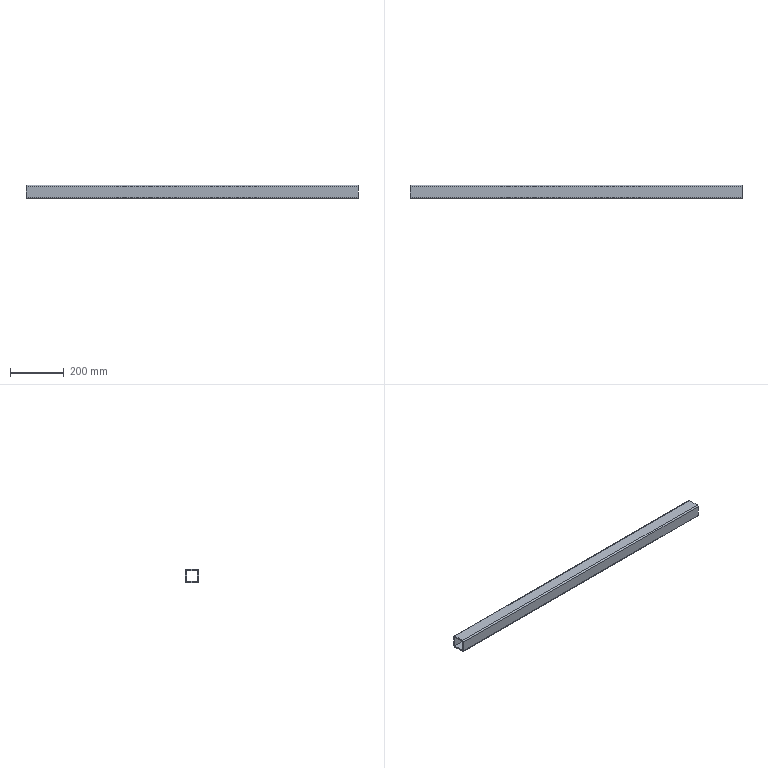Part | STEP file | 50x50x1240 | 1 solid | 14 faces | box 1240 x 50 x 50 mm | volume 1089389 mm3 | plane 10 | cylinder 4 | commonest cylinder face diameters 10 x4
STEP:
#1=CARTESIAN_POINT('',(0.,0.,0.));
#2=DIRECTION('',(0.,0.,1.));
#3=DIRECTION('',(1.,0.,0.));
#4=AXIS2_PLACEMENT_3D('',#1,#2,#3);
#5=CARTESIAN_POINT('',(-803.5,420.,-65.));
#6=VERTEX_POINT('',#5);
#7=CARTESIAN_POINT('',(-803.5,420.,-25.));
#8=VERTEX_POINT('',#7);
#9=CARTESIAN_POINT('',(-803.5,420.,-25.));
#10=DIRECTION('',(0.,0.,1.));
#11=VECTOR('',#10,1.);
#12=LINE('',#9,#11);
#13=CARTESIAN_POINT('',(636.5,420.,-25.));
#14=DIRECTION('',(0.,-1.,0.));
#15=DIRECTION('',(0.,0.,1.));
#16=AXIS2_PLACEMENT_3D('',#13,#14,#15);
#17=PLANE('',#16);
#18=CARTESIAN_POINT('',(0.,1440.));
#19=DIRECTION('',(1.,0.));
#20=VECTOR('',#19,1.);
#21=LINE('',#18,#20);
#22=(GEOMETRIC_REPRESENTATION_CONTEXT(2)PARAMETRIC_REPRESENTATION_CONTEXT()REPRESENTATION_CONTEXT('',''));
#23=DEFINITIONAL_REPRESENTATION('',(#21),#22);
#24=PCURVE('',#17,#23);
#25=CARTESIAN_POINT('',(-803.5,375.,-20.));
#26=DIRECTION('',(-1.,0.,0.));
#27=DIRECTION('',(0.,0.,1.));
#28=AXIS2_PLACEMENT_3D('',#25,#26,#27);
#29=PLANE('',#28);
#30=CARTESIAN_POINT('',(-5.,45.));
#31=DIRECTION('',(1.,0.));
#32=VECTOR('',#31,1.);
#33=LINE('',#30,#32);
#34=(GEOMETRIC_REPRESENTATION_CONTEXT(2)PARAMETRIC_REPRESENTATION_CONTEXT()REPRESENTATION_CONTEXT('',''));
#35=DEFINITIONAL_REPRESENTATION('',(#33),#34);
#36=PCURVE('',#29,#35);
#37=SURFACE_CURVE('',#12,(#24,#36),.PCURVE_S1.);
#38=EDGE_CURVE('',#6,#8,#37,.T.);
#39=ORIENTED_EDGE('',*,*,#38,.F.);
#40=CARTESIAN_POINT('',(436.5,420.,-65.));
#41=VERTEX_POINT('',#40);
#42=CARTESIAN_POINT('',(636.5,420.,-65.));
#43=DIRECTION('',(1.,0.,0.));
#44=VECTOR('',#43,1.);
#45=LINE('',#42,#44);
#46=CARTESIAN_POINT('',(-40.,0.));
#47=DIRECTION('',(0.,-1.));
#48=VECTOR('',#47,1.);
#49=LINE('',#46,#48);
#50=(GEOMETRIC_REPRESENTATION_CONTEXT(2)PARAMETRIC_REPRESENTATION_CONTEXT()REPRESENTATION_CONTEXT('',''));
#51=DEFINITIONAL_REPRESENTATION('',(#49),#50);
#52=PCURVE('',#17,#51);
#53=CARTESIAN_POINT('',(636.5,420.,-65.));
#54=DIRECTION('',(0.,0.,1.));
#55=DIRECTION('',(0.,1.,0.));
#56=AXIS2_PLACEMENT_3D('',#53,#54,#55);
#57=PLANE('',#56);
#58=CARTESIAN_POINT('',(0.,0.));
#59=DIRECTION('',(0.,-1.));
#60=VECTOR('',#59,1.);
#61=LINE('',#58,#60);
#62=(GEOMETRIC_REPRESENTATION_CONTEXT(2)PARAMETRIC_REPRESENTATION_CONTEXT()REPRESENTATION_CONTEXT('',''));
#63=DEFINITIONAL_REPRESENTATION('',(#61),#62);
#64=PCURVE('',#57,#63);
#65=SURFACE_CURVE('',#45,(#52,#64),.PCURVE_S1.);
#66=EDGE_CURVE('',#6,#41,#65,.T.);
#67=ORIENTED_EDGE('',*,*,#66,.T.);
#68=CARTESIAN_POINT('',(436.5,420.,-25.));
#69=VERTEX_POINT('',#68);
#70=CARTESIAN_POINT('',(436.5,420.,-25.));
#71=DIRECTION('',(0.,0.,1.));
#72=VECTOR('',#71,1.);
#73=LINE('',#70,#72);
#74=CARTESIAN_POINT('',(0.,200.));
#75=DIRECTION('',(1.,0.));
#76=VECTOR('',#75,1.);
#77=LINE('',#74,#76);
#78=(GEOMETRIC_REPRESENTATION_CONTEXT(2)PARAMETRIC_REPRESENTATION_CONTEXT()REPRESENTATION_CONTEXT('',''));
#79=DEFINITIONAL_REPRESENTATION('',(#77),#78);
#80=PCURVE('',#17,#79);
#81=CARTESIAN_POINT('',(436.5,420.,-670.));
#82=DIRECTION('',(-1.,0.,0.));
#83=DIRECTION('',(0.,0.,1.));
#84=AXIS2_PLACEMENT_3D('',#81,#82,#83);
#85=PLANE('',#84);
#86=CARTESIAN_POINT('',(645.,0.));
#87=DIRECTION('',(1.,0.));
#88=VECTOR('',#87,1.);
#89=LINE('',#86,#88);
#90=(GEOMETRIC_REPRESENTATION_CONTEXT(2)PARAMETRIC_REPRESENTATION_CONTEXT()REPRESENTATION_CONTEXT('',''));
#91=DEFINITIONAL_REPRESENTATION('',(#89),#90);
#92=PCURVE('',#85,#91);
#93=SURFACE_CURVE('',#73,(#80,#92),.PCURVE_S1.);
#94=EDGE_CURVE('',#41,#69,#93,.T.);
#95=ORIENTED_EDGE('',*,*,#94,.T.);
#96=CARTESIAN_POINT('',(636.5,420.,-25.));
#97=DIRECTION('',(1.,0.,0.));
#98=VECTOR('',#97,1.);
#99=LINE('',#96,#98);
#100=CARTESIAN_POINT('',(0.,0.));
#101=DIRECTION('',(0.,-1.));
#102=VECTOR('',#101,1.);
#103=LINE('',#100,#102);
#104=(GEOMETRIC_REPRESENTATION_CONTEXT(2)PARAMETRIC_REPRESENTATION_CONTEXT()REPRESENTATION_CONTEXT('',''));
#105=DEFINITIONAL_REPRESENTATION('',(#103),#104);
#106=PCURVE('',#17,#105);
#107=CARTESIAN_POINT('',(636.5,380.,-25.));
#108=DIRECTION('',(0.,0.,-1.));
#109=DIRECTION('',(0.,-1.,0.));
#110=AXIS2_PLACEMENT_3D('',#107,#108,#109);
#111=PLANE('',#110);
#112=CARTESIAN_POINT('',(-40.,0.));
#113=DIRECTION('',(0.,-1.));
#114=VECTOR('',#113,1.);
#115=LINE('',#112,#114);
#116=(GEOMETRIC_REPRESENTATION_CONTEXT(2)PARAMETRIC_REPRESENTATION_CONTEXT()REPRESENTATION_CONTEXT('',''));
#117=DEFINITIONAL_REPRESENTATION('',(#115),#116);
#118=PCURVE('',#111,#117);
#119=SURFACE_CURVE('',#99,(#106,#118),.PCURVE_S1.);
#120=EDGE_CURVE('',#8,#69,#119,.T.);
#121=ORIENTED_EDGE('',*,*,#120,.F.);
#122=EDGE_LOOP('',(#39,#67,#95,#121));
#123=FACE_BOUND('',#122,.T.);
#124=ADVANCED_FACE('',(#123),#17,.T.);
#125=CARTESIAN_POINT('',(-803.5,380.,-25.));
#126=VERTEX_POINT('',#125);
#127=CARTESIAN_POINT('',(-803.5,380.,-25.));
#128=DIRECTION('',(0.,-1.,0.));
#129=VECTOR('',#128,1.);
#130=LINE('',#127,#129);
#131=CARTESIAN_POINT('',(0.,1440.));
#132=DIRECTION('',(1.,0.));
#133=VECTOR('',#132,1.);
#134=LINE('',#131,#133);
#135=(GEOMETRIC_REPRESENTATION_CONTEXT(2)PARAMETRIC_REPRESENTATION_CONTEXT()REPRESENTATION_CONTEXT('',''));
#136=DEFINITIONAL_REPRESENTATION('',(#134),#135);
#137=PCURVE('',#111,#136);
#138=CARTESIAN_POINT('',(-5.,5.));
#139=DIRECTION('',(0.,-1.));
#140=VECTOR('',#139,1.);
#141=LINE('',#138,#140);
#142=(GEOMETRIC_REPRESENTATION_CONTEXT(2)PARAMETRIC_REPRESENTATION_CONTEXT()REPRESENTATION_CONTEXT('',''));
#143=DEFINITIONAL_REPRESENTATION('',(#141),#142);
#144=PCURVE('',#29,#143);
#145=SURFACE_CURVE('',#130,(#137,#144),.PCURVE_S1.);
#146=EDGE_CURVE('',#8,#126,#145,.T.);
#147=ORIENTED_EDGE('',*,*,#146,.F.);
#148=ORIENTED_EDGE('',*,*,#120,.T.);
#149=CARTESIAN_POINT('',(436.5,380.,-25.));
#150=VERTEX_POINT('',#149);
#151=CARTESIAN_POINT('',(436.5,380.,-25.));
#152=DIRECTION('',(0.,-1.,0.));
#153=VECTOR('',#152,1.);
#154=LINE('',#151,#153);
#155=CARTESIAN_POINT('',(0.,200.));
#156=DIRECTION('',(1.,0.));
#157=VECTOR('',#156,1.);
#158=LINE('',#155,#157);
#159=(GEOMETRIC_REPRESENTATION_CONTEXT(2)PARAMETRIC_REPRESENTATION_CONTEXT()REPRESENTATION_CONTEXT('',''));
#160=DEFINITIONAL_REPRESENTATION('',(#158),#159);
#161=PCURVE('',#111,#160);
#162=CARTESIAN_POINT('',(645.,-40.));
#163=DIRECTION('',(0.,-1.));
#164=VECTOR('',#163,1.);
#165=LINE('',#162,#164);
#166=(GEOMETRIC_REPRESENTATION_CONTEXT(2)PARAMETRIC_REPRESENTATION_CONTEXT()REPRESENTATION_CONTEXT('',''));
#167=DEFINITIONAL_REPRESENTATION('',(#165),#166);
#168=PCURVE('',#85,#167);
#169=SURFACE_CURVE('',#154,(#161,#168),.PCURVE_S1.);
#170=EDGE_CURVE('',#69,#150,#169,.T.);
#171=ORIENTED_EDGE('',*,*,#170,.T.);
#172=CARTESIAN_POINT('',(636.5,380.,-25.));
#173=DIRECTION('',(1.,0.,0.));
#174=VECTOR('',#173,1.);
#175=LINE('',#172,#174);
#176=CARTESIAN_POINT('',(0.,0.));
#177=DIRECTION('',(0.,-1.));
#178=VECTOR('',#177,1.);
#179=LINE('',#176,#178);
#180=(GEOMETRIC_REPRESENTATION_CONTEXT(2)PARAMETRIC_REPRESENTATION_CONTEXT()REPRESENTATION_CONTEXT('',''));
#181=DEFINITIONAL_REPRESENTATION('',(#179),#180);
#182=PCURVE('',#111,#181);
#183=CARTESIAN_POINT('',(636.5,380.,-65.));
#184=DIRECTION('',(0.,1.,0.));
#185=DIRECTION('',(0.,0.,-1.));
#186=AXIS2_PLACEMENT_3D('',#183,#184,#185);
#187=PLANE('',#186);
#188=CARTESIAN_POINT('',(-40.,0.));
#189=DIRECTION('',(0.,-1.));
#190=VECTOR('',#189,1.);
#191=LINE('',#188,#190);
#192=(GEOMETRIC_REPRESENTATION_CONTEXT(2)PARAMETRIC_REPRESENTATION_CONTEXT()REPRESENTATION_CONTEXT('',''));
#193=DEFINITIONAL_REPRESENTATION('',(#191),#192);
#194=PCURVE('',#187,#193);
#195=SURFACE_CURVE('',#175,(#182,#194),.PCURVE_S1.);
#196=EDGE_CURVE('',#126,#150,#195,.T.);
#197=ORIENTED_EDGE('',*,*,#196,.F.);
#198=EDGE_LOOP('',(#147,#148,#171,#197));
#199=FACE_BOUND('',#198,.T.);
#200=ADVANCED_FACE('',(#199),#111,.T.);
#201=CARTESIAN_POINT('',(-803.5,380.,-65.));
#202=VERTEX_POINT('',#201);
#203=CARTESIAN_POINT('',(-803.5,380.,-65.));
#204=DIRECTION('',(0.,0.,-1.));
#205=VECTOR('',#204,1.);
#206=LINE('',#203,#205);
#207=CARTESIAN_POINT('',(0.,1440.));
#208=DIRECTION('',(1.,0.));
#209=VECTOR('',#208,1.);
#210=LINE('',#207,#209);
#211=(GEOMETRIC_REPRESENTATION_CONTEXT(2)PARAMETRIC_REPRESENTATION_CONTEXT()REPRESENTATION_CONTEXT('',''));
#212=DEFINITIONAL_REPRESENTATION('',(#210),#211);
#213=PCURVE('',#187,#212);
#214=CARTESIAN_POINT('',(-45.,5.));
#215=DIRECTION('',(-1.,0.));
#216=VECTOR('',#215,1.);
#217=LINE('',#214,#216);
#218=(GEOMETRIC_REPRESENTATION_CONTEXT(2)PARAMETRIC_REPRESENTATION_CONTEXT()REPRESENTATION_CONTEXT('',''));
#219=DEFINITIONAL_REPRESENTATION('',(#217),#218);
#220=PCURVE('',#29,#219);
#221=SURFACE_CURVE('',#206,(#213,#220),.PCURVE_S1.);
#222=EDGE_CURVE('',#126,#202,#221,.T.);
#223=ORIENTED_EDGE('',*,*,#222,.F.);
#224=ORIENTED_EDGE('',*,*,#196,.T.);
#225=CARTESIAN_POINT('',(436.5,380.,-65.));
#226=VERTEX_POINT('',#225);
#227=CARTESIAN_POINT('',(436.5,380.,-65.));
#228=DIRECTION('',(0.,0.,-1.));
#229=VECTOR('',#228,1.);
#230=LINE('',#227,#229);
#231=CARTESIAN_POINT('',(0.,200.));
#232=DIRECTION('',(1.,0.));
#233=VECTOR('',#232,1.);
#234=LINE('',#231,#233);
#235=(GEOMETRIC_REPRESENTATION_CONTEXT(2)PARAMETRIC_REPRESENTATION_CONTEXT()REPRESENTATION_CONTEXT('',''));
#236=DEFINITIONAL_REPRESENTATION('',(#234),#235);
#237=PCURVE('',#187,#236);
#238=CARTESIAN_POINT('',(605.,-40.));
#239=DIRECTION('',(-1.,0.));
#240=VECTOR('',#239,1.);
#241=LINE('',#238,#240);
#242=(GEOMETRIC_REPRESENTATION_CONTEXT(2)PARAMETRIC_REPRESENTATION_CONTEXT()REPRESENTATION_CONTEXT('',''));
#243=DEFINITIONAL_REPRESENTATION('',(#241),#242);
#244=PCURVE('',#85,#243);
#245=SURFACE_CURVE('',#230,(#237,#244),.PCURVE_S1.);
#246=EDGE_CURVE('',#150,#226,#245,.T.);
#247=ORIENTED_EDGE('',*,*,#246,.T.);
#248=CARTESIAN_POINT('',(636.5,380.,-65.));
#249=DIRECTION('',(1.,0.,0.));
#250=VECTOR('',#249,1.);
#251=LINE('',#248,#250);
#252=CARTESIAN_POINT('',(0.,0.));
#253=DIRECTION('',(0.,-1.));
#254=VECTOR('',#253,1.);
#255=LINE('',#252,#254);
#256=(GEOMETRIC_REPRESENTATION_CONTEXT(2)PARAMETRIC_REPRESENTATION_CONTEXT()REPRESENTATION_CONTEXT('',''));
#257=DEFINITIONAL_REPRESENTATION('',(#255),#256);
#258=PCURVE('',#187,#257);
#259=CARTESIAN_POINT('',(-40.,0.));
#260=DIRECTION('',(0.,-1.));
#261=VECTOR('',#260,1.);
#262=LINE('',#259,#261);
#263=(GEOMETRIC_REPRESENTATION_CONTEXT(2)PARAMETRIC_REPRESENTATION_CONTEXT()REPRESENTATION_CONTEXT('',''));
#264=DEFINITIONAL_REPRESENTATION('',(#262),#263);
#265=PCURVE('',#57,#264);
#266=SURFACE_CURVE('',#251,(#258,#265),.PCURVE_S1.);
#267=EDGE_CURVE('',#202,#226,#266,.T.);
#268=ORIENTED_EDGE('',*,*,#267,.F.);
#269=EDGE_LOOP('',(#223,#224,#247,#268));
#270=FACE_BOUND('',#269,.T.);
#271=ADVANCED_FACE('',(#270),#187,.T.);
#272=CARTESIAN_POINT('',(-803.5,425.,-65.));
#273=VERTEX_POINT('',#272);
#274=CARTESIAN_POINT('',(-803.5,425.,-25.));
#275=VERTEX_POINT('',#274);
#276=CARTESIAN_POINT('',(-803.5,425.,-25.));
#277=DIRECTION('',(0.,0.,1.));
#278=VECTOR('',#277,1.);
#279=LINE('',#276,#278);
#280=CARTESIAN_POINT('',(636.5,425.,-25.));
#281=DIRECTION('',(0.,-1.,0.));
#282=DIRECTION('',(0.,0.,1.));
#283=AXIS2_PLACEMENT_3D('',#280,#281,#282);
#284=PLANE('',#283);
#285=CARTESIAN_POINT('',(0.,1440.));
#286=DIRECTION('',(1.,0.));
#287=VECTOR('',#286,1.);
#288=LINE('',#285,#287);
#289=(GEOMETRIC_REPRESENTATION_CONTEXT(2)PARAMETRIC_REPRESENTATION_CONTEXT()REPRESENTATION_CONTEXT('',''));
#290=DEFINITIONAL_REPRESENTATION('',(#288),#289);
#291=PCURVE('',#284,#290);
#292=CARTESIAN_POINT('',(-5.,50.));
#293=DIRECTION('',(1.,0.));
#294=VECTOR('',#293,1.);
#295=LINE('',#292,#294);
#296=(GEOMETRIC_REPRESENTATION_CONTEXT(2)PARAMETRIC_REPRESENTATION_CONTEXT()REPRESENTATION_CONTEXT('',''));
#297=DEFINITIONAL_REPRESENTATION('',(#295),#296);
#298=PCURVE('',#29,#297);
#299=SURFACE_CURVE('',#279,(#291,#298),.PCURVE_S1.);
#300=EDGE_CURVE('',#273,#275,#299,.T.);
#301=ORIENTED_EDGE('',*,*,#300,.T.);
#302=CARTESIAN_POINT('',(436.5,425.,-25.));
#303=VERTEX_POINT('',#302);
#304=CARTESIAN_POINT('',(636.5,425.,-25.));
#305=DIRECTION('',(1.,0.,0.));
#306=VECTOR('',#305,1.);
#307=LINE('',#304,#306);
#308=CARTESIAN_POINT('',(0.,0.));
#309=DIRECTION('',(0.,-1.));
#310=VECTOR('',#309,1.);
#311=LINE('',#308,#310);
#312=(GEOMETRIC_REPRESENTATION_CONTEXT(2)PARAMETRIC_REPRESENTATION_CONTEXT()REPRESENTATION_CONTEXT('',''));
#313=DEFINITIONAL_REPRESENTATION('',(#311),#312);
#314=PCURVE('',#284,#313);
#315=CARTESIAN_POINT('',(636.5,420.,-25.));
#316=DIRECTION('',(-1.,0.,0.));
#317=DIRECTION('',(0.,0.,1.));
#318=AXIS2_PLACEMENT_3D('',#315,#316,#317);
#319=CYLINDRICAL_SURFACE('',#318,5.);
#320=CARTESIAN_POINT('',(1.571,0.));
#321=DIRECTION('',(0.,-1.));
#322=VECTOR('',#321,1.);
#323=LINE('',#320,#322);
#324=(GEOMETRIC_REPRESENTATION_CONTEXT(2)PARAMETRIC_REPRESENTATION_CONTEXT()REPRESENTATION_CONTEXT('',''));
#325=DEFINITIONAL_REPRESENTATION('',(#323),#324);
#326=PCURVE('',#319,#325);
#327=SURFACE_CURVE('',#307,(#314,#326),.PCURVE_S1.);
#328=EDGE_CURVE('',#275,#303,#327,.T.);
#329=ORIENTED_EDGE('',*,*,#328,.T.);
#330=CARTESIAN_POINT('',(436.5,425.,-65.));
#331=VERTEX_POINT('',#330);
#332=CARTESIAN_POINT('',(436.5,425.,-25.));
#333=DIRECTION('',(0.,0.,1.));
#334=VECTOR('',#333,1.);
#335=LINE('',#332,#334);
#336=CARTESIAN_POINT('',(0.,200.));
#337=DIRECTION('',(1.,0.));
#338=VECTOR('',#337,1.);
#339=LINE('',#336,#338);
#340=(GEOMETRIC_REPRESENTATION_CONTEXT(2)PARAMETRIC_REPRESENTATION_CONTEXT()REPRESENTATION_CONTEXT('',''));
#341=DEFINITIONAL_REPRESENTATION('',(#339),#340);
#342=PCURVE('',#284,#341);
#343=CARTESIAN_POINT('',(645.,5.));
#344=DIRECTION('',(1.,0.));
#345=VECTOR('',#344,1.);
#346=LINE('',#343,#345);
#347=(GEOMETRIC_REPRESENTATION_CONTEXT(2)PARAMETRIC_REPRESENTATION_CONTEXT()REPRESENTATION_CONTEXT('',''));
#348=DEFINITIONAL_REPRESENTATION('',(#346),#347);
#349=PCURVE('',#85,#348);
#350=SURFACE_CURVE('',#335,(#342,#349),.PCURVE_S1.);
#351=EDGE_CURVE('',#331,#303,#350,.T.);
#352=ORIENTED_EDGE('',*,*,#351,.F.);
#353=CARTESIAN_POINT('',(636.5,425.,-65.));
#354=DIRECTION('',(1.,0.,0.));
#355=VECTOR('',#354,1.);
#356=LINE('',#353,#355);
#357=CARTESIAN_POINT('',(-40.,0.));
#358=DIRECTION('',(0.,-1.));
#359=VECTOR('',#358,1.);
#360=LINE('',#357,#359);
#361=(GEOMETRIC_REPRESENTATION_CONTEXT(2)PARAMETRIC_REPRESENTATION_CONTEXT()REPRESENTATION_CONTEXT('',''));
#362=DEFINITIONAL_REPRESENTATION('',(#360),#361);
#363=PCURVE('',#284,#362);
#364=CARTESIAN_POINT('',(636.5,420.,-65.));
#365=DIRECTION('',(-1.,0.,0.));
#366=DIRECTION('',(0.,0.,1.));
#367=AXIS2_PLACEMENT_3D('',#364,#365,#366);
#368=CYLINDRICAL_SURFACE('',#367,5.);
#369=CARTESIAN_POINT('',(1.571,0.));
#370=DIRECTION('',(0.,-1.));
#371=VECTOR('',#370,1.);
#372=LINE('',#369,#371);
#373=(GEOMETRIC_REPRESENTATION_CONTEXT(2)PARAMETRIC_REPRESENTATION_CONTEXT()REPRESENTATION_CONTEXT('',''));
#374=DEFINITIONAL_REPRESENTATION('',(#372),#373);
#375=PCURVE('',#368,#374);
#376=SURFACE_CURVE('',#356,(#363,#375),.PCURVE_S1.);
#377=EDGE_CURVE('',#273,#331,#376,.T.);
#378=ORIENTED_EDGE('',*,*,#377,.F.);
#379=EDGE_LOOP('',(#301,#329,#352,#378));
#380=FACE_BOUND('',#379,.T.);
#381=ADVANCED_FACE('',(#380),#284,.F.);
#382=CARTESIAN_POINT('',(-803.5,420.,-70.));
#383=VERTEX_POINT('',#382);
#384=CARTESIAN_POINT('',(-803.5,420.,-65.));
#385=DIRECTION('',(1.,0.,0.));
#386=DIRECTION('',(0.,0.,1.));
#387=AXIS2_PLACEMENT_3D('',#384,#385,#386);
#388=CIRCLE('',#387,5.);
#389=CARTESIAN_POINT('',(6.283,1440.));
#390=DIRECTION('',(-1.,0.));
#391=VECTOR('',#390,1.);
#392=LINE('',#389,#391);
#393=(GEOMETRIC_REPRESENTATION_CONTEXT(2)PARAMETRIC_REPRESENTATION_CONTEXT()REPRESENTATION_CONTEXT('',''));
#394=DEFINITIONAL_REPRESENTATION('',(#392),#393);
#395=PCURVE('',#368,#394);
#396=CARTESIAN_POINT('',(-40.,45.));
#397=CARTESIAN_POINT('',(-40.,36.34));
#398=CARTESIAN_POINT('',(-47.5,40.67));
#399=CARTESIAN_POINT('',(-55.,45.));
#400=CARTESIAN_POINT('',(-47.5,49.33));
#401=CARTESIAN_POINT('',(-40.,53.66));
#402=CARTESIAN_POINT('',(-40.,45.));
#403=(BOUNDED_CURVE()B_SPLINE_CURVE(2,(#396,#397,#398,#399,#400,#401,#402),.UNSPECIFIED.,.T.,.F.)B_SPLINE_CURVE_WITH_KNOTS((1,2,2,2,2,1),(-2.094,0.,2.094,4.189,6.283,8.378),.UNSPECIFIED.)CURVE()GEOMETRIC_REPRESENTATION_ITEM()RATIONAL_B_SPLINE_CURVE((1.,0.5,1.,0.5,1.,0.5,1.))REPRESENTATION_ITEM(''));
#404=(GEOMETRIC_REPRESENTATION_CONTEXT(2)PARAMETRIC_REPRESENTATION_CONTEXT()REPRESENTATION_CONTEXT('',''));
#405=DEFINITIONAL_REPRESENTATION('',(#403),#404);
#406=PCURVE('',#29,#405);
#407=SURFACE_CURVE('',#388,(#395,#406),.PCURVE_S1.);
#408=EDGE_CURVE('',#383,#273,#407,.T.);
#409=ORIENTED_EDGE('',*,*,#408,.T.);
#410=ORIENTED_EDGE('',*,*,#377,.T.);
#411=CARTESIAN_POINT('',(436.5,420.,-70.));
#412=VERTEX_POINT('',#411);
#413=CARTESIAN_POINT('',(436.5,420.,-65.));
#414=DIRECTION('',(1.,0.,0.));
#415=DIRECTION('',(0.,0.,1.));
#416=AXIS2_PLACEMENT_3D('',#413,#414,#415);
#417=CIRCLE('',#416,5.);
#418=CARTESIAN_POINT('',(6.283,200.));
#419=DIRECTION('',(-1.,0.));
#420=VECTOR('',#419,1.);
#421=LINE('',#418,#420);
#422=(GEOMETRIC_REPRESENTATION_CONTEXT(2)PARAMETRIC_REPRESENTATION_CONTEXT()REPRESENTATION_CONTEXT('',''));
#423=DEFINITIONAL_REPRESENTATION('',(#421),#422);
#424=PCURVE('',#368,#423);
#425=CARTESIAN_POINT('',(610.,0.));
#426=CARTESIAN_POINT('',(610.,-8.66));
#427=CARTESIAN_POINT('',(602.5,-4.33));
#428=CARTESIAN_POINT('',(595.,0.));
#429=CARTESIAN_POINT('',(602.5,4.33));
#430=CARTESIAN_POINT('',(610.,8.66));
#431=CARTESIAN_POINT('',(610.,0.));
#432=(BOUNDED_CURVE()B_SPLINE_CURVE(2,(#425,#426,#427,#428,#429,#430,#431),.UNSPECIFIED.,.T.,.F.)B_SPLINE_CURVE_WITH_KNOTS((1,2,2,2,2,1),(-2.094,0.,2.094,4.189,6.283,8.378),.UNSPECIFIED.)CURVE()GEOMETRIC_REPRESENTATION_ITEM()RATIONAL_B_SPLINE_CURVE((1.,0.5,1.,0.5,1.,0.5,1.))REPRESENTATION_ITEM(''));
#433=(GEOMETRIC_REPRESENTATION_CONTEXT(2)PARAMETRIC_REPRESENTATION_CONTEXT()REPRESENTATION_CONTEXT('',''));
#434=DEFINITIONAL_REPRESENTATION('',(#432),#433);
#435=PCURVE('',#85,#434);
#436=SURFACE_CURVE('',#417,(#424,#435),.PCURVE_S1.);
#437=EDGE_CURVE('',#412,#331,#436,.T.);
#438=ORIENTED_EDGE('',*,*,#437,.F.);
#439=CARTESIAN_POINT('',(636.5,420.,-70.));
#440=DIRECTION('',(1.,0.,0.));
#441=VECTOR('',#440,1.);
#442=LINE('',#439,#441);
#443=CARTESIAN_POINT('',(3.142,0.));
#444=DIRECTION('',(0.,-1.));
#445=VECTOR('',#444,1.);
#446=LINE('',#443,#445);
#447=(GEOMETRIC_REPRESENTATION_CONTEXT(2)PARAMETRIC_REPRESENTATION_CONTEXT()REPRESENTATION_CONTEXT('',''));
#448=DEFINITIONAL_REPRESENTATION('',(#446),#447);
#449=PCURVE('',#368,#448);
#450=CARTESIAN_POINT('',(636.5,420.,-70.));
#451=DIRECTION('',(0.,0.,1.));
#452=DIRECTION('',(0.,1.,0.));
#453=AXIS2_PLACEMENT_3D('',#450,#451,#452);
#454=PLANE('',#453);
#455=CARTESIAN_POINT('',(0.,0.));
#456=DIRECTION('',(0.,-1.));
#457=VECTOR('',#456,1.);
#458=LINE('',#455,#457);
#459=(GEOMETRIC_REPRESENTATION_CONTEXT(2)PARAMETRIC_REPRESENTATION_CONTEXT()REPRESENTATION_CONTEXT('',''));
#460=DEFINITIONAL_REPRESENTATION('',(#458),#459);
#461=PCURVE('',#454,#460);
#462=SURFACE_CURVE('',#442,(#449,#461),.PCURVE_S1.);
#463=EDGE_CURVE('',#383,#412,#462,.T.);
#464=ORIENTED_EDGE('',*,*,#463,.F.);
#465=EDGE_LOOP('',(#409,#410,#438,#464));
#466=FACE_BOUND('',#465,.T.);
#467=ADVANCED_FACE('',(#466),#368,.T.);
#468=CARTESIAN_POINT('',(-803.5,380.,-70.));
#469=VERTEX_POINT('',#468);
#470=CARTESIAN_POINT('',(-803.5,420.,-70.));
#471=DIRECTION('',(0.,1.,0.));
#472=VECTOR('',#471,1.);
#473=LINE('',#470,#472);
#474=CARTESIAN_POINT('',(0.,1440.));
#475=DIRECTION('',(1.,0.));
#476=VECTOR('',#475,1.);
#477=LINE('',#474,#476);
#478=(GEOMETRIC_REPRESENTATION_CONTEXT(2)PARAMETRIC_REPRESENTATION_CONTEXT()REPRESENTATION_CONTEXT('',''));
#479=DEFINITIONAL_REPRESENTATION('',(#477),#478);
#480=PCURVE('',#454,#479);
#481=CARTESIAN_POINT('',(-50.,45.));
#482=DIRECTION('',(0.,1.));
#483=VECTOR('',#482,1.);
#484=LINE('',#481,#483);
#485=(GEOMETRIC_REPRESENTATION_CONTEXT(2)PARAMETRIC_REPRESENTATION_CONTEXT()REPRESENTATION_CONTEXT('',''));
#486=DEFINITIONAL_REPRESENTATION('',(#484),#485);
#487=PCURVE('',#29,#486);
#488=SURFACE_CURVE('',#473,(#480,#487),.PCURVE_S1.);
#489=EDGE_CURVE('',#469,#383,#488,.T.);
#490=ORIENTED_EDGE('',*,*,#489,.T.);
#491=ORIENTED_EDGE('',*,*,#463,.T.);
#492=CARTESIAN_POINT('',(436.5,380.,-70.));
#493=VERTEX_POINT('',#492);
#494=CARTESIAN_POINT('',(436.5,420.,-70.));
#495=DIRECTION('',(0.,1.,0.));
#496=VECTOR('',#495,1.);
#497=LINE('',#494,#496);
#498=CARTESIAN_POINT('',(0.,200.));
#499=DIRECTION('',(1.,0.));
#500=VECTOR('',#499,1.);
#501=LINE('',#498,#500);
#502=(GEOMETRIC_REPRESENTATION_CONTEXT(2)PARAMETRIC_REPRESENTATION_CONTEXT()REPRESENTATION_CONTEXT('',''));
#503=DEFINITIONAL_REPRESENTATION('',(#501),#502);
#504=PCURVE('',#454,#503);
#505=CARTESIAN_POINT('',(600.,0.));
#506=DIRECTION('',(0.,1.));
#507=VECTOR('',#506,1.);
#508=LINE('',#505,#507);
#509=(GEOMETRIC_REPRESENTATION_CONTEXT(2)PARAMETRIC_REPRESENTATION_CONTEXT()REPRESENTATION_CONTEXT('',''));
#510=DEFINITIONAL_REPRESENTATION('',(#508),#509);
#511=PCURVE('',#85,#510);
#512=SURFACE_CURVE('',#497,(#504,#511),.PCURVE_S1.);
#513=EDGE_CURVE('',#493,#412,#512,.T.);
#514=ORIENTED_EDGE('',*,*,#513,.F.);
#515=CARTESIAN_POINT('',(636.5,380.,-70.));
#516=DIRECTION('',(1.,0.,0.));
#517=VECTOR('',#516,1.);
#518=LINE('',#515,#517);
#519=CARTESIAN_POINT('',(-40.,0.));
#520=DIRECTION('',(0.,-1.));
#521=VECTOR('',#520,1.);
#522=LINE('',#519,#521);
#523=(GEOMETRIC_REPRESENTATION_CONTEXT(2)PARAMETRIC_REPRESENTATION_CONTEXT()REPRESENTATION_CONTEXT('',''));
#524=DEFINITIONAL_REPRESENTATION('',(#522),#523);
#525=PCURVE('',#454,#524);
#526=CARTESIAN_POINT('',(636.5,380.,-65.));
#527=DIRECTION('',(-1.,0.,0.));
#528=DIRECTION('',(0.,0.,1.));
#529=AXIS2_PLACEMENT_3D('',#526,#527,#528);
#530=CYLINDRICAL_SURFACE('',#529,5.);
#531=CARTESIAN_POINT('',(3.142,0.));
#532=DIRECTION('',(0.,-1.));
#533=VECTOR('',#532,1.);
#534=LINE('',#531,#533);
#535=(GEOMETRIC_REPRESENTATION_CONTEXT(2)PARAMETRIC_REPRESENTATION_CONTEXT()REPRESENTATION_CONTEXT('',''));
#536=DEFINITIONAL_REPRESENTATION('',(#534),#535);
#537=PCURVE('',#530,#536);
#538=SURFACE_CURVE('',#518,(#525,#537),.PCURVE_S1.);
#539=EDGE_CURVE('',#469,#493,#538,.T.);
#540=ORIENTED_EDGE('',*,*,#539,.F.);
#541=EDGE_LOOP('',(#490,#491,#514,#540));
#542=FACE_BOUND('',#541,.T.);
#543=ADVANCED_FACE('',(#542),#454,.F.);
#544=CARTESIAN_POINT('',(-803.5,375.,-65.));
#545=VERTEX_POINT('',#544);
#546=CARTESIAN_POINT('',(-803.5,380.,-65.));
#547=DIRECTION('',(1.,0.,0.));
#548=DIRECTION('',(0.,0.,1.));
#549=AXIS2_PLACEMENT_3D('',#546,#547,#548);
#550=CIRCLE('',#549,5.);
#551=CARTESIAN_POINT('',(6.283,1440.));
#552=DIRECTION('',(-1.,0.));
#553=VECTOR('',#552,1.);
#554=LINE('',#551,#553);
#555=(GEOMETRIC_REPRESENTATION_CONTEXT(2)PARAMETRIC_REPRESENTATION_CONTEXT()REPRESENTATION_CONTEXT('',''));
#556=DEFINITIONAL_REPRESENTATION('',(#554),#555);
#557=PCURVE('',#530,#556);
#558=CARTESIAN_POINT('',(-40.,5.));
#559=CARTESIAN_POINT('',(-40.,-3.66));
#560=CARTESIAN_POINT('',(-47.5,0.6699));
#561=CARTESIAN_POINT('',(-55.,5.));
#562=CARTESIAN_POINT('',(-47.5,9.33));
#563=CARTESIAN_POINT('',(-40.,13.66));
#564=CARTESIAN_POINT('',(-40.,5.));
#565=(BOUNDED_CURVE()B_SPLINE_CURVE(2,(#558,#559,#560,#561,#562,#563,#564),.UNSPECIFIED.,.T.,.F.)B_SPLINE_CURVE_WITH_KNOTS((1,2,2,2,2,1),(-2.094,0.,2.094,4.189,6.283,8.378),.UNSPECIFIED.)CURVE()GEOMETRIC_REPRESENTATION_ITEM()RATIONAL_B_SPLINE_CURVE((1.,0.5,1.,0.5,1.,0.5,1.))REPRESENTATION_ITEM(''));
#566=(GEOMETRIC_REPRESENTATION_CONTEXT(2)PARAMETRIC_REPRESENTATION_CONTEXT()REPRESENTATION_CONTEXT('',''));
#567=DEFINITIONAL_REPRESENTATION('',(#565),#566);
#568=PCURVE('',#29,#567);
#569=SURFACE_CURVE('',#550,(#557,#568),.PCURVE_S1.);
#570=EDGE_CURVE('',#545,#469,#569,.T.);
#571=ORIENTED_EDGE('',*,*,#570,.T.);
#572=ORIENTED_EDGE('',*,*,#539,.T.);
#573=CARTESIAN_POINT('',(436.5,375.,-65.));
#574=VERTEX_POINT('',#573);
#575=CARTESIAN_POINT('',(436.5,380.,-65.));
#576=DIRECTION('',(1.,0.,0.));
#577=DIRECTION('',(0.,0.,1.));
#578=AXIS2_PLACEMENT_3D('',#575,#576,#577);
#579=CIRCLE('',#578,5.);
#580=CARTESIAN_POINT('',(6.283,200.));
#581=DIRECTION('',(-1.,0.));
#582=VECTOR('',#581,1.);
#583=LINE('',#580,#582);
#584=(GEOMETRIC_REPRESENTATION_CONTEXT(2)PARAMETRIC_REPRESENTATION_CONTEXT()REPRESENTATION_CONTEXT('',''));
#585=DEFINITIONAL_REPRESENTATION('',(#583),#584);
#586=PCURVE('',#530,#585);
#587=CARTESIAN_POINT('',(610.,-40.));
#588=CARTESIAN_POINT('',(610.,-48.66));
#589=CARTESIAN_POINT('',(602.5,-44.33));
#590=CARTESIAN_POINT('',(595.,-40.));
#591=CARTESIAN_POINT('',(602.5,-35.67));
#592=CARTESIAN_POINT('',(610.,-31.34));
#593=CARTESIAN_POINT('',(610.,-40.));
#594=(BOUNDED_CURVE()B_SPLINE_CURVE(2,(#587,#588,#589,#590,#591,#592,#593),.UNSPECIFIED.,.T.,.F.)B_SPLINE_CURVE_WITH_KNOTS((1,2,2,2,2,1),(-2.094,0.,2.094,4.189,6.283,8.378),.UNSPECIFIED.)CURVE()GEOMETRIC_REPRESENTATION_ITEM()RATIONAL_B_SPLINE_CURVE((1.,0.5,1.,0.5,1.,0.5,1.))REPRESENTATION_ITEM(''));
#595=(GEOMETRIC_REPRESENTATION_CONTEXT(2)PARAMETRIC_REPRESENTATION_CONTEXT()REPRESENTATION_CONTEXT('',''));
#596=DEFINITIONAL_REPRESENTATION('',(#594),#595);
#597=PCURVE('',#85,#596);
#598=SURFACE_CURVE('',#579,(#586,#597),.PCURVE_S1.);
#599=EDGE_CURVE('',#574,#493,#598,.T.);
#600=ORIENTED_EDGE('',*,*,#599,.F.);
#601=CARTESIAN_POINT('',(636.5,375.,-65.));
#602=DIRECTION('',(1.,0.,0.));
#603=VECTOR('',#602,1.);
#604=LINE('',#601,#603);
#605=CARTESIAN_POINT('',(4.712,0.));
#606=DIRECTION('',(0.,-1.));
#607=VECTOR('',#606,1.);
#608=LINE('',#605,#607);
#609=(GEOMETRIC_REPRESENTATION_CONTEXT(2)PARAMETRIC_REPRESENTATION_CONTEXT()REPRESENTATION_CONTEXT('',''));
#610=DEFINITIONAL_REPRESENTATION('',(#608),#609);
#611=PCURVE('',#530,#610);
#612=CARTESIAN_POINT('',(636.5,375.,-65.));
#613=DIRECTION('',(0.,1.,0.));
#614=DIRECTION('',(0.,0.,-1.));
#615=AXIS2_PLACEMENT_3D('',#612,#613,#614);
#616=PLANE('',#615);
#617=CARTESIAN_POINT('',(0.,0.));
#618=DIRECTION('',(0.,-1.));
#619=VECTOR('',#618,1.);
#620=LINE('',#617,#619);
#621=(GEOMETRIC_REPRESENTATION_CONTEXT(2)PARAMETRIC_REPRESENTATION_CONTEXT()REPRESENTATION_CONTEXT('',''));
#622=DEFINITIONAL_REPRESENTATION('',(#620),#621);
#623=PCURVE('',#616,#622);
#624=SURFACE_CURVE('',#604,(#611,#623),.PCURVE_S1.);
#625=EDGE_CURVE('',#545,#574,#624,.T.);
#626=ORIENTED_EDGE('',*,*,#625,.F.);
#627=EDGE_LOOP('',(#571,#572,#600,#626));
#628=FACE_BOUND('',#627,.T.);
#629=ADVANCED_FACE('',(#628),#530,.T.);
#630=CARTESIAN_POINT('',(-803.5,375.,-25.));
#631=VERTEX_POINT('',#630);
#632=CARTESIAN_POINT('',(-803.5,375.,-65.));
#633=DIRECTION('',(0.,0.,-1.));
#634=VECTOR('',#633,1.);
#635=LINE('',#632,#634);
#636=CARTESIAN_POINT('',(0.,1440.));
#637=DIRECTION('',(1.,0.));
#638=VECTOR('',#637,1.);
#639=LINE('',#636,#638);
#640=(GEOMETRIC_REPRESENTATION_CONTEXT(2)PARAMETRIC_REPRESENTATION_CONTEXT()REPRESENTATION_CONTEXT('',''));
#641=DEFINITIONAL_REPRESENTATION('',(#639),#640);
#642=PCURVE('',#616,#641);
#643=CARTESIAN_POINT('',(-45.,0.));
#644=DIRECTION('',(-1.,0.));
#645=VECTOR('',#644,1.);
#646=LINE('',#643,#645);
#647=(GEOMETRIC_REPRESENTATION_CONTEXT(2)PARAMETRIC_REPRESENTATION_CONTEXT()REPRESENTATION_CONTEXT('',''));
#648=DEFINITIONAL_REPRESENTATION('',(#646),#647);
#649=PCURVE('',#29,#648);
#650=SURFACE_CURVE('',#635,(#642,#649),.PCURVE_S1.);
#651=EDGE_CURVE('',#631,#545,#650,.T.);
#652=ORIENTED_EDGE('',*,*,#651,.T.);
#653=ORIENTED_EDGE('',*,*,#625,.T.);
#654=CARTESIAN_POINT('',(436.5,375.,-25.));
#655=VERTEX_POINT('',#654);
#656=CARTESIAN_POINT('',(436.5,375.,-65.));
#657=DIRECTION('',(0.,0.,-1.));
#658=VECTOR('',#657,1.);
#659=LINE('',#656,#658);
#660=CARTESIAN_POINT('',(0.,200.));
#661=DIRECTION('',(1.,0.));
#662=VECTOR('',#661,1.);
#663=LINE('',#660,#662);
#664=(GEOMETRIC_REPRESENTATION_CONTEXT(2)PARAMETRIC_REPRESENTATION_CONTEXT()REPRESENTATION_CONTEXT('',''));
#665=DEFINITIONAL_REPRESENTATION('',(#663),#664);
#666=PCURVE('',#616,#665);
#667=CARTESIAN_POINT('',(605.,-45.));
#668=DIRECTION('',(-1.,0.));
#669=VECTOR('',#668,1.);
#670=LINE('',#667,#669);
#671=(GEOMETRIC_REPRESENTATION_CONTEXT(2)PARAMETRIC_REPRESENTATION_CONTEXT()REPRESENTATION_CONTEXT('',''));
#672=DEFINITIONAL_REPRESENTATION('',(#670),#671);
#673=PCURVE('',#85,#672);
#674=SURFACE_CURVE('',#659,(#666,#673),.PCURVE_S1.);
#675=EDGE_CURVE('',#655,#574,#674,.T.);
#676=ORIENTED_EDGE('',*,*,#675,.F.);
#677=CARTESIAN_POINT('',(636.5,375.,-25.));
#678=DIRECTION('',(1.,0.,0.));
#679=VECTOR('',#678,1.);
#680=LINE('',#677,#679);
#681=CARTESIAN_POINT('',(-40.,0.));
#682=DIRECTION('',(0.,-1.));
#683=VECTOR('',#682,1.);
#684=LINE('',#681,#683);
#685=(GEOMETRIC_REPRESENTATION_CONTEXT(2)PARAMETRIC_REPRESENTATION_CONTEXT()REPRESENTATION_CONTEXT('',''));
#686=DEFINITIONAL_REPRESENTATION('',(#684),#685);
#687=PCURVE('',#616,#686);
#688=CARTESIAN_POINT('',(636.5,380.,-25.));
#689=DIRECTION('',(-1.,0.,0.));
#690=DIRECTION('',(0.,0.,1.));
#691=AXIS2_PLACEMENT_3D('',#688,#689,#690);
#692=CYLINDRICAL_SURFACE('',#691,5.);
#693=CARTESIAN_POINT('',(4.712,0.));
#694=DIRECTION('',(0.,-1.));
#695=VECTOR('',#694,1.);
#696=LINE('',#693,#695);
#697=(GEOMETRIC_REPRESENTATION_CONTEXT(2)PARAMETRIC_REPRESENTATION_CONTEXT()REPRESENTATION_CONTEXT('',''));
#698=DEFINITIONAL_REPRESENTATION('',(#696),#697);
#699=PCURVE('',#692,#698);
#700=SURFACE_CURVE('',#680,(#687,#699),.PCURVE_S1.);
#701=EDGE_CURVE('',#631,#655,#700,.T.);
#702=ORIENTED_EDGE('',*,*,#701,.F.);
#703=EDGE_LOOP('',(#652,#653,#676,#702));
#704=FACE_BOUND('',#703,.T.);
#705=ADVANCED_FACE('',(#704),#616,.F.);
#706=CARTESIAN_POINT('',(-803.5,380.,-20.));
#707=VERTEX_POINT('',#706);
#708=CARTESIAN_POINT('',(-803.5,380.,-25.));
#709=DIRECTION('',(1.,0.,0.));
#710=DIRECTION('',(0.,0.,1.));
#711=AXIS2_PLACEMENT_3D('',#708,#709,#710);
#712=CIRCLE('',#711,5.);
#713=CARTESIAN_POINT('',(6.283,1440.));
#714=DIRECTION('',(-1.,0.));
#715=VECTOR('',#714,1.);
#716=LINE('',#713,#715);
#717=(GEOMETRIC_REPRESENTATION_CONTEXT(2)PARAMETRIC_REPRESENTATION_CONTEXT()REPRESENTATION_CONTEXT('',''));
#718=DEFINITIONAL_REPRESENTATION('',(#716),#717);
#719=PCURVE('',#692,#718);
#720=CARTESIAN_POINT('',(0.,5.));
#721=CARTESIAN_POINT('',(0.,-3.66));
#722=CARTESIAN_POINT('',(-7.5,0.6699));
#723=CARTESIAN_POINT('',(-15.,5.));
#724=CARTESIAN_POINT('',(-7.5,9.33));
#725=CARTESIAN_POINT('',(0.,13.66));
#726=CARTESIAN_POINT('',(0.,5.));
#727=(BOUNDED_CURVE()B_SPLINE_CURVE(2,(#720,#721,#722,#723,#724,#725,#726),.UNSPECIFIED.,.T.,.F.)B_SPLINE_CURVE_WITH_KNOTS((1,2,2,2,2,1),(-2.094,0.,2.094,4.189,6.283,8.378),.UNSPECIFIED.)CURVE()GEOMETRIC_REPRESENTATION_ITEM()RATIONAL_B_SPLINE_CURVE((1.,0.5,1.,0.5,1.,0.5,1.))REPRESENTATION_ITEM(''));
#728=(GEOMETRIC_REPRESENTATION_CONTEXT(2)PARAMETRIC_REPRESENTATION_CONTEXT()REPRESENTATION_CONTEXT('',''));
#729=DEFINITIONAL_REPRESENTATION('',(#727),#728);
#730=PCURVE('',#29,#729);
#731=SURFACE_CURVE('',#712,(#719,#730),.PCURVE_S1.);
#732=EDGE_CURVE('',#707,#631,#731,.T.);
#733=ORIENTED_EDGE('',*,*,#732,.T.);
#734=ORIENTED_EDGE('',*,*,#701,.T.);
#735=CARTESIAN_POINT('',(436.5,380.,-20.));
#736=VERTEX_POINT('',#735);
#737=CARTESIAN_POINT('',(436.5,380.,-25.));
#738=DIRECTION('',(1.,0.,0.));
#739=DIRECTION('',(0.,0.,1.));
#740=AXIS2_PLACEMENT_3D('',#737,#738,#739);
#741=CIRCLE('',#740,5.);
#742=CARTESIAN_POINT('',(6.283,200.));
#743=DIRECTION('',(-1.,0.));
#744=VECTOR('',#743,1.);
#745=LINE('',#742,#744);
#746=(GEOMETRIC_REPRESENTATION_CONTEXT(2)PARAMETRIC_REPRESENTATION_CONTEXT()REPRESENTATION_CONTEXT('',''));
#747=DEFINITIONAL_REPRESENTATION('',(#745),#746);
#748=PCURVE('',#692,#747);
#749=CARTESIAN_POINT('',(650.,-40.));
#750=CARTESIAN_POINT('',(650.,-48.66));
#751=CARTESIAN_POINT('',(642.5,-44.33));
#752=CARTESIAN_POINT('',(635.,-40.));
#753=CARTESIAN_POINT('',(642.5,-35.67));
#754=CARTESIAN_POINT('',(650.,-31.34));
#755=CARTESIAN_POINT('',(650.,-40.));
#756=(BOUNDED_CURVE()B_SPLINE_CURVE(2,(#749,#750,#751,#752,#753,#754,#755),.UNSPECIFIED.,.T.,.F.)B_SPLINE_CURVE_WITH_KNOTS((1,2,2,2,2,1),(-2.094,0.,2.094,4.189,6.283,8.378),.UNSPECIFIED.)CURVE()GEOMETRIC_REPRESENTATION_ITEM()RATIONAL_B_SPLINE_CURVE((1.,0.5,1.,0.5,1.,0.5,1.))REPRESENTATION_ITEM(''));
#757=(GEOMETRIC_REPRESENTATION_CONTEXT(2)PARAMETRIC_REPRESENTATION_CONTEXT()REPRESENTATION_CONTEXT('',''));
#758=DEFINITIONAL_REPRESENTATION('',(#756),#757);
#759=PCURVE('',#85,#758);
#760=SURFACE_CURVE('',#741,(#748,#759),.PCURVE_S1.);
#761=EDGE_CURVE('',#736,#655,#760,.T.);
#762=ORIENTED_EDGE('',*,*,#761,.F.);
#763=CARTESIAN_POINT('',(636.5,380.,-20.));
#764=DIRECTION('',(1.,0.,0.));
#765=VECTOR('',#764,1.);
#766=LINE('',#763,#765);
#767=CARTESIAN_POINT('',(6.283,0.));
#768=DIRECTION('',(0.,-1.));
#769=VECTOR('',#768,1.);
#770=LINE('',#767,#769);
#771=(GEOMETRIC_REPRESENTATION_CONTEXT(2)PARAMETRIC_REPRESENTATION_CONTEXT()REPRESENTATION_CONTEXT('',''));
#772=DEFINITIONAL_REPRESENTATION('',(#770),#771);
#773=PCURVE('',#692,#772);
#774=CARTESIAN_POINT('',(636.5,380.,-20.));
#775=DIRECTION('',(0.,0.,-1.));
#776=DIRECTION('',(0.,-1.,0.));
#777=AXIS2_PLACEMENT_3D('',#774,#775,#776);
#778=PLANE('',#777);
#779=CARTESIAN_POINT('',(0.,0.));
#780=DIRECTION('',(0.,-1.));
#781=VECTOR('',#780,1.);
#782=LINE('',#779,#781);
#783=(GEOMETRIC_REPRESENTATION_CONTEXT(2)PARAMETRIC_REPRESENTATION_CONTEXT()REPRESENTATION_CONTEXT('',''));
#784=DEFINITIONAL_REPRESENTATION('',(#782),#783);
#785=PCURVE('',#778,#784);
#786=SURFACE_CURVE('',#766,(#773,#785),.PCURVE_S1.);
#787=EDGE_CURVE('',#707,#736,#786,.T.);
#788=ORIENTED_EDGE('',*,*,#787,.F.);
#789=EDGE_LOOP('',(#733,#734,#762,#788));
#790=FACE_BOUND('',#789,.T.);
#791=ADVANCED_FACE('',(#790),#692,.T.);
#792=CARTESIAN_POINT('',(-803.5,420.,-20.));
#793=VERTEX_POINT('',#792);
#794=CARTESIAN_POINT('',(-803.5,380.,-20.));
#795=DIRECTION('',(0.,-1.,0.));
#796=VECTOR('',#795,1.);
#797=LINE('',#794,#796);
#798=CARTESIAN_POINT('',(0.,1440.));
#799=DIRECTION('',(1.,0.));
#800=VECTOR('',#799,1.);
#801=LINE('',#798,#800);
#802=(GEOMETRIC_REPRESENTATION_CONTEXT(2)PARAMETRIC_REPRESENTATION_CONTEXT()REPRESENTATION_CONTEXT('',''));
#803=DEFINITIONAL_REPRESENTATION('',(#801),#802);
#804=PCURVE('',#778,#803);
#805=CARTESIAN_POINT('',(0.,5.));
#806=DIRECTION('',(0.,-1.));
#807=VECTOR('',#806,1.);
#808=LINE('',#805,#807);
#809=(GEOMETRIC_REPRESENTATION_CONTEXT(2)PARAMETRIC_REPRESENTATION_CONTEXT()REPRESENTATION_CONTEXT('',''));
#810=DEFINITIONAL_REPRESENTATION('',(#808),#809);
#811=PCURVE('',#29,#810);
#812=SURFACE_CURVE('',#797,(#804,#811),.PCURVE_S1.);
#813=EDGE_CURVE('',#793,#707,#812,.T.);
#814=ORIENTED_EDGE('',*,*,#813,.T.);
#815=ORIENTED_EDGE('',*,*,#787,.T.);
#816=CARTESIAN_POINT('',(436.5,420.,-20.));
#817=VERTEX_POINT('',#816);
#818=CARTESIAN_POINT('',(436.5,380.,-20.));
#819=DIRECTION('',(0.,-1.,0.));
#820=VECTOR('',#819,1.);
#821=LINE('',#818,#820);
#822=CARTESIAN_POINT('',(0.,200.));
#823=DIRECTION('',(1.,0.));
#824=VECTOR('',#823,1.);
#825=LINE('',#822,#824);
#826=(GEOMETRIC_REPRESENTATION_CONTEXT(2)PARAMETRIC_REPRESENTATION_CONTEXT()REPRESENTATION_CONTEXT('',''));
#827=DEFINITIONAL_REPRESENTATION('',(#825),#826);
#828=PCURVE('',#778,#827);
#829=CARTESIAN_POINT('',(650.,-40.));
#830=DIRECTION('',(0.,-1.));
#831=VECTOR('',#830,1.);
#832=LINE('',#829,#831);
#833=(GEOMETRIC_REPRESENTATION_CONTEXT(2)PARAMETRIC_REPRESENTATION_CONTEXT()REPRESENTATION_CONTEXT('',''));
#834=DEFINITIONAL_REPRESENTATION('',(#832),#833);
#835=PCURVE('',#85,#834);
#836=SURFACE_CURVE('',#821,(#828,#835),.PCURVE_S1.);
#837=EDGE_CURVE('',#817,#736,#836,.T.);
#838=ORIENTED_EDGE('',*,*,#837,.F.);
#839=CARTESIAN_POINT('',(636.5,420.,-20.));
#840=DIRECTION('',(1.,0.,0.));
#841=VECTOR('',#840,1.);
#842=LINE('',#839,#841);
#843=CARTESIAN_POINT('',(-40.,0.));
#844=DIRECTION('',(0.,-1.));
#845=VECTOR('',#844,1.);
#846=LINE('',#843,#845);
#847=(GEOMETRIC_REPRESENTATION_CONTEXT(2)PARAMETRIC_REPRESENTATION_CONTEXT()REPRESENTATION_CONTEXT('',''));
#848=DEFINITIONAL_REPRESENTATION('',(#846),#847);
#849=PCURVE('',#778,#848);
#850=CARTESIAN_POINT('',(0.,0.));
#851=DIRECTION('',(0.,-1.));
#852=VECTOR('',#851,1.);
#853=LINE('',#850,#852);
#854=(GEOMETRIC_REPRESENTATION_CONTEXT(2)PARAMETRIC_REPRESENTATION_CONTEXT()REPRESENTATION_CONTEXT('',''));
#855=DEFINITIONAL_REPRESENTATION('',(#853),#854);
#856=PCURVE('',#319,#855);
#857=SURFACE_CURVE('',#842,(#849,#856),.PCURVE_S1.);
#858=EDGE_CURVE('',#793,#817,#857,.T.);
#859=ORIENTED_EDGE('',*,*,#858,.F.);
#860=EDGE_LOOP('',(#814,#815,#838,#859));
#861=FACE_BOUND('',#860,.T.);
#862=ADVANCED_FACE('',(#861),#778,.F.);
#863=CARTESIAN_POINT('',(-803.5,420.,-25.));
#864=DIRECTION('',(1.,0.,0.));
#865=DIRECTION('',(0.,0.,1.));
#866=AXIS2_PLACEMENT_3D('',#863,#864,#865);
#867=CIRCLE('',#866,5.);
#868=CARTESIAN_POINT('',(6.283,1440.));
#869=DIRECTION('',(-1.,0.));
#870=VECTOR('',#869,1.);
#871=LINE('',#868,#870);
#872=(GEOMETRIC_REPRESENTATION_CONTEXT(2)PARAMETRIC_REPRESENTATION_CONTEXT()REPRESENTATION_CONTEXT('',''));
#873=DEFINITIONAL_REPRESENTATION('',(#871),#872);
#874=PCURVE('',#319,#873);
#875=CARTESIAN_POINT('',(0.,45.));
#876=CARTESIAN_POINT('',(0.,36.34));
#877=CARTESIAN_POINT('',(-7.5,40.67));
#878=CARTESIAN_POINT('',(-15.,45.));
#879=CARTESIAN_POINT('',(-7.5,49.33));
#880=CARTESIAN_POINT('',(0.,53.66));
#881=CARTESIAN_POINT('',(0.,45.));
#882=(BOUNDED_CURVE()B_SPLINE_CURVE(2,(#875,#876,#877,#878,#879,#880,#881),.UNSPECIFIED.,.T.,.F.)B_SPLINE_CURVE_WITH_KNOTS((1,2,2,2,2,1),(-2.094,0.,2.094,4.189,6.283,8.378),.UNSPECIFIED.)CURVE()GEOMETRIC_REPRESENTATION_ITEM()RATIONAL_B_SPLINE_CURVE((1.,0.5,1.,0.5,1.,0.5,1.))REPRESENTATION_ITEM(''));
#883=(GEOMETRIC_REPRESENTATION_CONTEXT(2)PARAMETRIC_REPRESENTATION_CONTEXT()REPRESENTATION_CONTEXT('',''));
#884=DEFINITIONAL_REPRESENTATION('',(#882),#883);
#885=PCURVE('',#29,#884);
#886=SURFACE_CURVE('',#867,(#874,#885),.PCURVE_S1.);
#887=EDGE_CURVE('',#275,#793,#886,.T.);
#888=ORIENTED_EDGE('',*,*,#887,.T.);
#889=ORIENTED_EDGE('',*,*,#858,.T.);
#890=CARTESIAN_POINT('',(436.5,420.,-25.));
#891=DIRECTION('',(1.,0.,0.));
#892=DIRECTION('',(0.,0.,1.));
#893=AXIS2_PLACEMENT_3D('',#890,#891,#892);
#894=CIRCLE('',#893,5.);
#895=CARTESIAN_POINT('',(6.283,200.));
#896=DIRECTION('',(-1.,0.));
#897=VECTOR('',#896,1.);
#898=LINE('',#895,#897);
#899=(GEOMETRIC_REPRESENTATION_CONTEXT(2)PARAMETRIC_REPRESENTATION_CONTEXT()REPRESENTATION_CONTEXT('',''));
#900=DEFINITIONAL_REPRESENTATION('',(#898),#899);
#901=PCURVE('',#319,#900);
#902=CARTESIAN_POINT('',(650.,0.));
#903=CARTESIAN_POINT('',(650.,-8.66));
#904=CARTESIAN_POINT('',(642.5,-4.33));
#905=CARTESIAN_POINT('',(635.,0.));
#906=CARTESIAN_POINT('',(642.5,4.33));
#907=CARTESIAN_POINT('',(650.,8.66));
#908=CARTESIAN_POINT('',(650.,0.));
#909=(BOUNDED_CURVE()B_SPLINE_CURVE(2,(#902,#903,#904,#905,#906,#907,#908),.UNSPECIFIED.,.T.,.F.)B_SPLINE_CURVE_WITH_KNOTS((1,2,2,2,2,1),(-2.094,0.,2.094,4.189,6.283,8.378),.UNSPECIFIED.)CURVE()GEOMETRIC_REPRESENTATION_ITEM()RATIONAL_B_SPLINE_CURVE((1.,0.5,1.,0.5,1.,0.5,1.))REPRESENTATION_ITEM(''));
#910=(GEOMETRIC_REPRESENTATION_CONTEXT(2)PARAMETRIC_REPRESENTATION_CONTEXT()REPRESENTATION_CONTEXT('',''));
#911=DEFINITIONAL_REPRESENTATION('',(#909),#910);
#912=PCURVE('',#85,#911);
#913=SURFACE_CURVE('',#894,(#901,#912),.PCURVE_S1.);
#914=EDGE_CURVE('',#303,#817,#913,.T.);
#915=ORIENTED_EDGE('',*,*,#914,.F.);
#916=ORIENTED_EDGE('',*,*,#328,.F.);
#917=EDGE_LOOP('',(#888,#889,#915,#916));
#918=FACE_BOUND('',#917,.T.);
#919=ADVANCED_FACE('',(#918),#319,.T.);
#920=CARTESIAN_POINT('',(-803.5,420.,-65.));
#921=DIRECTION('',(0.,1.,0.));
#922=VECTOR('',#921,1.);
#923=LINE('',#920,#922);
#924=CARTESIAN_POINT('',(0.,1440.));
#925=DIRECTION('',(1.,0.));
#926=VECTOR('',#925,1.);
#927=LINE('',#924,#926);
#928=(GEOMETRIC_REPRESENTATION_CONTEXT(2)PARAMETRIC_REPRESENTATION_CONTEXT()REPRESENTATION_CONTEXT('',''));
#929=DEFINITIONAL_REPRESENTATION('',(#927),#928);
#930=PCURVE('',#57,#929);
#931=CARTESIAN_POINT('',(-45.,45.));
#932=DIRECTION('',(0.,1.));
#933=VECTOR('',#932,1.);
#934=LINE('',#931,#933);
#935=(GEOMETRIC_REPRESENTATION_CONTEXT(2)PARAMETRIC_REPRESENTATION_CONTEXT()REPRESENTATION_CONTEXT('',''));
#936=DEFINITIONAL_REPRESENTATION('',(#934),#935);
#937=PCURVE('',#29,#936);
#938=SURFACE_CURVE('',#923,(#930,#937),.PCURVE_S1.);
#939=EDGE_CURVE('',#202,#6,#938,.T.);
#940=ORIENTED_EDGE('',*,*,#939,.F.);
#941=ORIENTED_EDGE('',*,*,#267,.T.);
#942=CARTESIAN_POINT('',(436.5,420.,-65.));
#943=DIRECTION('',(0.,1.,0.));
#944=VECTOR('',#943,1.);
#945=LINE('',#942,#944);
#946=CARTESIAN_POINT('',(0.,200.));
#947=DIRECTION('',(1.,0.));
#948=VECTOR('',#947,1.);
#949=LINE('',#946,#948);
#950=(GEOMETRIC_REPRESENTATION_CONTEXT(2)PARAMETRIC_REPRESENTATION_CONTEXT()REPRESENTATION_CONTEXT('',''));
#951=DEFINITIONAL_REPRESENTATION('',(#949),#950);
#952=PCURVE('',#57,#951);
#953=CARTESIAN_POINT('',(605.,0.));
#954=DIRECTION('',(0.,1.));
#955=VECTOR('',#954,1.);
#956=LINE('',#953,#955);
#957=(GEOMETRIC_REPRESENTATION_CONTEXT(2)PARAMETRIC_REPRESENTATION_CONTEXT()REPRESENTATION_CONTEXT('',''));
#958=DEFINITIONAL_REPRESENTATION('',(#956),#957);
#959=PCURVE('',#85,#958);
#960=SURFACE_CURVE('',#945,(#952,#959),.PCURVE_S1.);
#961=EDGE_CURVE('',#226,#41,#960,.T.);
#962=ORIENTED_EDGE('',*,*,#961,.T.);
#963=ORIENTED_EDGE('',*,*,#66,.F.);
#964=EDGE_LOOP('',(#940,#941,#962,#963));
#965=FACE_BOUND('',#964,.T.);
#966=ADVANCED_FACE('',(#965),#57,.T.);
#967=ORIENTED_EDGE('',*,*,#351,.T.);
#968=ORIENTED_EDGE('',*,*,#914,.T.);
#969=ORIENTED_EDGE('',*,*,#837,.T.);
#970=ORIENTED_EDGE('',*,*,#761,.T.);
#971=ORIENTED_EDGE('',*,*,#675,.T.);
#972=ORIENTED_EDGE('',*,*,#599,.T.);
#973=ORIENTED_EDGE('',*,*,#513,.T.);
#974=ORIENTED_EDGE('',*,*,#437,.T.);
#975=EDGE_LOOP('',(#967,#968,#969,#970,#971,#972,#973,#974));
#976=FACE_BOUND('',#975,.T.);
#977=ORIENTED_EDGE('',*,*,#94,.F.);
#978=ORIENTED_EDGE('',*,*,#961,.F.);
#979=ORIENTED_EDGE('',*,*,#246,.F.);
#980=ORIENTED_EDGE('',*,*,#170,.F.);
#981=EDGE_LOOP('',(#977,#978,#979,#980));
#982=FACE_BOUND('',#981,.T.);
#983=ADVANCED_FACE('',(#976,#982),#85,.F.);
#984=ORIENTED_EDGE('',*,*,#300,.F.);
#985=ORIENTED_EDGE('',*,*,#408,.F.);
#986=ORIENTED_EDGE('',*,*,#489,.F.);
#987=ORIENTED_EDGE('',*,*,#570,.F.);
#988=ORIENTED_EDGE('',*,*,#651,.F.);
#989=ORIENTED_EDGE('',*,*,#732,.F.);
#990=ORIENTED_EDGE('',*,*,#813,.F.);
#991=ORIENTED_EDGE('',*,*,#887,.F.);
#992=EDGE_LOOP('',(#984,#985,#986,#987,#988,#989,#990,#991));
#993=FACE_BOUND('',#992,.T.);
#994=ORIENTED_EDGE('',*,*,#38,.T.);
#995=ORIENTED_EDGE('',*,*,#146,.T.);
#996=ORIENTED_EDGE('',*,*,#222,.T.);
#997=ORIENTED_EDGE('',*,*,#939,.T.);
#998=EDGE_LOOP('',(#994,#995,#996,#997));
#999=FACE_BOUND('',#998,.T.);
#1000=ADVANCED_FACE('',(#993,#999),#29,.T.);
#1001=CLOSED_SHELL('',(#124,#200,#271,#381,#467,#543,#629,#705,#791,#862,#919,#966,#983,#1000));
#1002=MANIFOLD_SOLID_BREP('',#1001);
#1003=(LENGTH_UNIT()NAMED_UNIT(*)SI_UNIT(.MILLI.,.METRE.));
#1004=UNCERTAINTY_MEASURE_WITH_UNIT(LENGTH_MEASURE(0.0000001),#1003,'','');
#1005=(NAMED_UNIT(*)PLANE_ANGLE_UNIT()SI_UNIT($,.RADIAN.));
#1006=(NAMED_UNIT(*)SI_UNIT($,.STERADIAN.)SOLID_ANGLE_UNIT());
#1007=(GEOMETRIC_REPRESENTATION_CONTEXT(3)GLOBAL_UNCERTAINTY_ASSIGNED_CONTEXT((#1004))GLOBAL_UNIT_ASSIGNED_CONTEXT((#1003,#1005,#1006))REPRESENTATION_CONTEXT('',''));
#1008=ADVANCED_BREP_SHAPE_REPRESENTATION('',(#4,#1002),#1007);